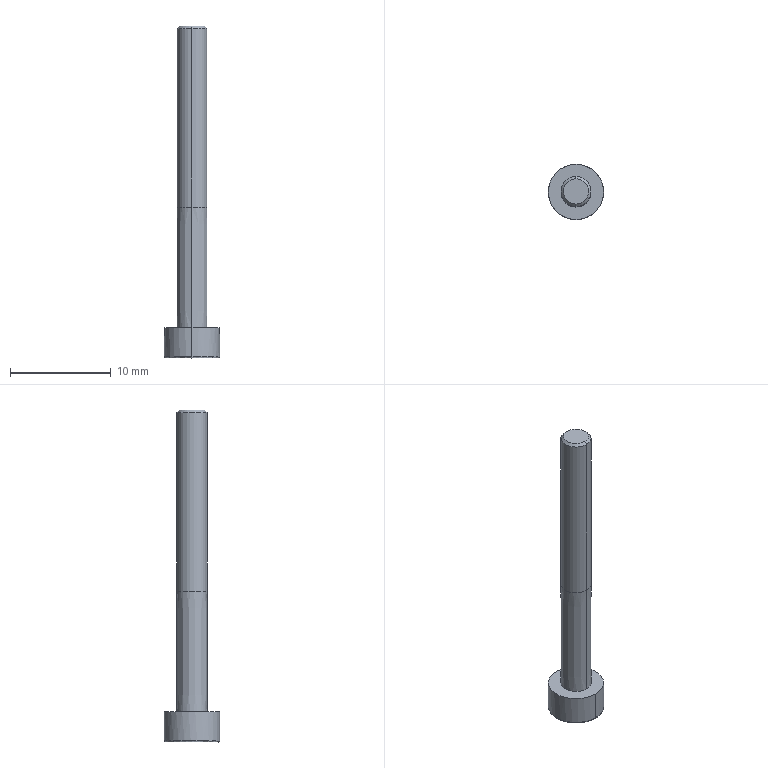Part | SolidWorks | features BaseBody 1 | 1 solid | 20 faces | box 5.5 x 5.5 x 33 mm | volume 275.938 mm3 | plane 10 | cylinder 4 | cone 4 | spline 2 | commonest cylinder face diameters 3 x2 5.5 x2
STEP:
#1=CARTESIAN_POINT('',(500.195,-28.804,245.644));
#2=VERTEX_POINT('',#1);
#3=CARTESIAN_POINT('',(502.224,-33.412,245.644));
#4=VERTEX_POINT('',#3);
#5=CARTESIAN_POINT('',(502.224,-30.662,245.644));
#6=DIRECTION('',(-0.000000001,-0.000000029,1.));
#7=DIRECTION('',(0.,-1.,-0.000000029));
#8=AXIS2_PLACEMENT_3D('',#5,#6,#7);
#9=CIRCLE('',#8,2.75);
#10=EDGE_CURVE('',#2,#4,#9,.T.);
#11=ORIENTED_EDGE('',*,*,#10,.F.);
#12=CARTESIAN_POINT('',(500.269,-28.872,245.544));
#13=VERTEX_POINT('',#12);
#14=CARTESIAN_POINT('',(500.269,-28.872,245.644));
#15=DIRECTION('',(-0.6753,-0.7375,-0.000000022));
#16=DIRECTION('',(-0.7375,0.6753,0.000000019));
#17=AXIS2_PLACEMENT_3D('',#14,#15,#16);
#18=CIRCLE('',#17,0.1);
#19=EDGE_CURVE('',#2,#13,#18,.T.);
#20=ORIENTED_EDGE('',*,*,#19,.T.);
#21=CARTESIAN_POINT('',(504.178,-32.451,245.544));
#22=VERTEX_POINT('',#21);
#23=CARTESIAN_POINT('',(500.269,-28.872,245.544));
#24=CARTESIAN_POINT('',(496.69,-32.781,245.544));
#25=CARTESIAN_POINT('',(500.599,-36.36,245.544));
#26=CARTESIAN_POINT('',(504.178,-32.451,245.544));
#27=(BOUNDED_CURVE()B_SPLINE_CURVE(3,(#23,#24,#25,#26),.UNSPECIFIED.,.F.,.F.)B_SPLINE_CURVE_WITH_KNOTS((4,4),(0.,1.),.UNSPECIFIED.)CURVE()GEOMETRIC_REPRESENTATION_ITEM()RATIONAL_B_SPLINE_CURVE((1.,0.3333,0.3333,1.))REPRESENTATION_ITEM(''));
#28=EDGE_CURVE('',#13,#22,#27,.T.);
#29=ORIENTED_EDGE('',*,*,#28,.T.);
#30=CARTESIAN_POINT('',(504.252,-32.519,245.644));
#31=VERTEX_POINT('',#30);
#32=CARTESIAN_POINT('',(504.178,-32.451,245.644));
#33=DIRECTION('',(0.6753,0.7375,0.000000022));
#34=DIRECTION('',(0.7375,-0.6753,-0.000000019));
#35=AXIS2_PLACEMENT_3D('',#32,#33,#34);
#36=CIRCLE('',#35,0.1);
#37=EDGE_CURVE('',#31,#22,#36,.T.);
#38=ORIENTED_EDGE('',*,*,#37,.F.);
#39=CARTESIAN_POINT('',(502.224,-30.662,245.644));
#40=DIRECTION('',(-0.000000001,-0.000000029,1.));
#41=DIRECTION('',(0.,-1.,-0.000000029));
#42=AXIS2_PLACEMENT_3D('',#39,#40,#41);
#43=CIRCLE('',#42,2.75);
#44=EDGE_CURVE('',#4,#31,#43,.T.);
#45=ORIENTED_EDGE('',*,*,#44,.F.);
#46=EDGE_LOOP('',(#11,#20,#29,#38,#45));
#47=FACE_OUTER_BOUND('',#46,.T.);
#48=CARTESIAN_POINT('',(500.195,-28.804,245.644));
#49=CARTESIAN_POINT('',(496.481,-32.861,245.644));
#50=CARTESIAN_POINT('',(500.537,-36.575,245.644));
#51=CARTESIAN_POINT('',(504.252,-32.519,245.644));
#52=CARTESIAN_POINT('',(500.195,-28.804,245.586));
#53=CARTESIAN_POINT('',(496.481,-32.861,245.586));
#54=CARTESIAN_POINT('',(500.537,-36.575,245.586));
#55=CARTESIAN_POINT('',(504.252,-32.519,245.586));
#56=CARTESIAN_POINT('',(500.226,-28.832,245.544));
#57=CARTESIAN_POINT('',(496.568,-32.828,245.544));
#58=CARTESIAN_POINT('',(500.563,-36.486,245.544));
#59=CARTESIAN_POINT('',(504.221,-32.491,245.544));
#60=CARTESIAN_POINT('',(500.269,-28.872,245.544));
#61=CARTESIAN_POINT('',(496.69,-32.781,245.544));
#62=CARTESIAN_POINT('',(500.599,-36.36,245.544));
#63=CARTESIAN_POINT('',(504.178,-32.451,245.544));
#64=(BOUNDED_SURFACE()B_SPLINE_SURFACE(3,3,((#48,#49,#50,#51),(#52,#53,#54,#55),(#56,#57,#58,#59),(#60,#61,#62,#63)),.UNSPECIFIED.,.F.,.F.,.F.)B_SPLINE_SURFACE_WITH_KNOTS((4,4),(4,4),(0.,1.),(0.,1.),.UNSPECIFIED.)GEOMETRIC_REPRESENTATION_ITEM()RATIONAL_B_SPLINE_SURFACE(((1.,0.3333,0.3333,1.),(0.8047,0.2682,0.2682,0.8047),(0.8047,0.2682,0.2682,0.8047),(1.,0.3333,0.3333,1.)))REPRESENTATION_ITEM('')SURFACE());
#65=ADVANCED_FACE('',(#47),#64,.T.);
#66=CARTESIAN_POINT('',(502.224,-32.162,260.544));
#67=VERTEX_POINT('',#66);
#68=CARTESIAN_POINT('',(502.224,-29.162,260.544));
#69=VERTEX_POINT('',#68);
#70=CARTESIAN_POINT('',(502.224,-30.662,260.544));
#71=DIRECTION('',(-0.000000001,-0.000000029,1.));
#72=DIRECTION('',(0.,-1.,-0.000000029));
#73=AXIS2_PLACEMENT_3D('',#70,#71,#72);
#74=CIRCLE('',#73,1.5);
#75=EDGE_CURVE('',#67,#69,#74,.T.);
#76=ORIENTED_EDGE('',*,*,#75,.T.);
#77=CARTESIAN_POINT('',(502.224,-29.162,278.294));
#78=VERTEX_POINT('',#77);
#79=CARTESIAN_POINT('',(502.224,-29.162,269.419));
#80=DIRECTION('',(-0.000000001,-0.000000029,1.));
#81=VECTOR('',#80,1000.);
#82=LINE('',#79,#81);
#83=EDGE_CURVE('',#69,#78,#82,.T.);
#84=ORIENTED_EDGE('',*,*,#83,.T.);
#85=CARTESIAN_POINT('',(502.224,-32.162,278.294));
#86=VERTEX_POINT('',#85);
#87=CARTESIAN_POINT('',(502.224,-30.662,278.294));
#88=DIRECTION('',(0.000000001,0.000000029,-1.));
#89=DIRECTION('',(0.,-1.,-0.000000029));
#90=AXIS2_PLACEMENT_3D('',#87,#88,#89);
#91=CIRCLE('',#90,1.5);
#92=EDGE_CURVE('',#78,#86,#91,.T.);
#93=ORIENTED_EDGE('',*,*,#92,.T.);
#94=CARTESIAN_POINT('',(502.224,-32.162,269.419));
#95=DIRECTION('',(-0.000000001,-0.000000029,1.));
#96=VECTOR('',#95,1000.);
#97=LINE('',#94,#96);
#98=EDGE_CURVE('',#67,#86,#97,.T.);
#99=ORIENTED_EDGE('',*,*,#98,.F.);
#100=EDGE_LOOP('',(#76,#84,#93,#99));
#101=FACE_OUTER_BOUND('',#100,.T.);
#102=CARTESIAN_POINT('',(502.224,-30.662,269.419));
#103=DIRECTION('',(-0.000000001,-0.000000029,1.));
#104=DIRECTION('',(0.,-1.,-0.000000029));
#105=AXIS2_PLACEMENT_3D('',#102,#103,#104);
#106=CYLINDRICAL_SURFACE('',#105,1.5);
#107=ADVANCED_FACE('',(#101),#106,.T.);
#108=CARTESIAN_POINT('',(502.224,-32.161,248.544));
#109=VERTEX_POINT('',#108);
#110=CARTESIAN_POINT('',(502.224,-29.162,248.544));
#111=VERTEX_POINT('',#110);
#112=CARTESIAN_POINT('',(502.224,-30.662,248.544));
#113=DIRECTION('',(-0.000000001,-0.000000029,1.));
#114=DIRECTION('',(0.,-1.,-0.000000029));
#115=AXIS2_PLACEMENT_3D('',#112,#113,#114);
#116=CIRCLE('',#115,1.499);
#117=EDGE_CURVE('',#109,#111,#116,.T.);
#118=ORIENTED_EDGE('',*,*,#117,.T.);
#119=CARTESIAN_POINT('',(502.224,-29.162,260.544));
#120=DIRECTION('',(-0.000000001,0.00006247,1.));
#121=VECTOR('',#120,1000.);
#122=LINE('',#119,#121);
#123=EDGE_CURVE('',#111,#69,#122,.T.);
#124=ORIENTED_EDGE('',*,*,#123,.T.);
#125=ORIENTED_EDGE('',*,*,#75,.F.);
#126=CARTESIAN_POINT('',(502.224,-32.162,260.544));
#127=DIRECTION('',(-0.000000001,-0.00006253,1.));
#128=VECTOR('',#127,1000.);
#129=LINE('',#126,#128);
#130=EDGE_CURVE('',#109,#67,#129,.T.);
#131=ORIENTED_EDGE('',*,*,#130,.F.);
#132=EDGE_LOOP('',(#118,#124,#125,#131));
#133=FACE_OUTER_BOUND('',#132,.T.);
#134=CARTESIAN_POINT('',(502.224,-30.662,260.544));
#135=DIRECTION('',(-0.000000001,-0.000000029,1.));
#136=DIRECTION('',(0.,-1.,-0.000000029));
#137=AXIS2_PLACEMENT_3D('',#134,#135,#136);
#138=CONICAL_SURFACE('',#137,1.5,0.0000625);
#139=ADVANCED_FACE('',(#133),#138,.T.);
#140=CARTESIAN_POINT('',(502.224,-29.412,278.544));
#141=VERTEX_POINT('',#140);
#142=CARTESIAN_POINT('',(502.224,-31.912,278.544));
#143=VERTEX_POINT('',#142);
#144=CARTESIAN_POINT('',(502.224,-30.662,278.544));
#145=DIRECTION('',(0.000000001,0.000000029,-1.));
#146=DIRECTION('',(0.,1.,0.000000029));
#147=AXIS2_PLACEMENT_3D('',#144,#145,#146);
#148=CIRCLE('',#147,1.25);
#149=EDGE_CURVE('',#141,#143,#148,.T.);
#150=ORIENTED_EDGE('',*,*,#149,.T.);
#151=CARTESIAN_POINT('',(502.224,-32.162,278.294));
#152=DIRECTION('',(0.,-0.7071,-0.7071));
#153=VECTOR('',#152,1000.);
#154=LINE('',#151,#153);
#155=EDGE_CURVE('',#143,#86,#154,.T.);
#156=ORIENTED_EDGE('',*,*,#155,.T.);
#157=ORIENTED_EDGE('',*,*,#92,.F.);
#158=CARTESIAN_POINT('',(502.224,-29.162,278.294));
#159=DIRECTION('',(0.,0.7071,-0.7071));
#160=VECTOR('',#159,1000.);
#161=LINE('',#158,#160);
#162=EDGE_CURVE('',#141,#78,#161,.T.);
#163=ORIENTED_EDGE('',*,*,#162,.F.);
#164=EDGE_LOOP('',(#150,#156,#157,#163));
#165=FACE_OUTER_BOUND('',#164,.T.);
#166=CARTESIAN_POINT('',(502.224,-30.662,278.294));
#167=DIRECTION('',(0.000000001,0.000000029,-1.));
#168=DIRECTION('',(0.,1.,0.000000029));
#169=AXIS2_PLACEMENT_3D('',#166,#167,#168);
#170=CONICAL_SURFACE('',#169,1.5,0.7854);
#171=ADVANCED_FACE('',(#165),#170,.T.);
#172=ORIENTED_EDGE('',*,*,#44,.T.);
#173=CARTESIAN_POINT('',(502.224,-27.912,245.644));
#174=VERTEX_POINT('',#173);
#175=CARTESIAN_POINT('',(502.224,-30.662,245.644));
#176=DIRECTION('',(-0.000000001,-0.000000029,1.));
#177=DIRECTION('',(0.,-1.,-0.000000029));
#178=AXIS2_PLACEMENT_3D('',#175,#176,#177);
#179=CIRCLE('',#178,2.75);
#180=EDGE_CURVE('',#31,#174,#179,.T.);
#181=ORIENTED_EDGE('',*,*,#180,.T.);
#182=CARTESIAN_POINT('',(502.224,-27.912,248.544));
#183=VERTEX_POINT('',#182);
#184=CARTESIAN_POINT('',(502.224,-27.912,247.094));
#185=DIRECTION('',(-0.000000001,-0.000000029,1.));
#186=VECTOR('',#185,1000.);
#187=LINE('',#184,#186);
#188=EDGE_CURVE('',#174,#183,#187,.T.);
#189=ORIENTED_EDGE('',*,*,#188,.T.);
#190=CARTESIAN_POINT('',(502.224,-33.412,248.544));
#191=VERTEX_POINT('',#190);
#192=CARTESIAN_POINT('',(502.224,-30.662,248.544));
#193=DIRECTION('',(-0.000000001,-0.000000029,1.));
#194=DIRECTION('',(0.,-1.,-0.000000029));
#195=AXIS2_PLACEMENT_3D('',#192,#193,#194);
#196=CIRCLE('',#195,2.75);
#197=EDGE_CURVE('',#191,#183,#196,.T.);
#198=ORIENTED_EDGE('',*,*,#197,.F.);
#199=CARTESIAN_POINT('',(502.224,-33.412,247.094));
#200=DIRECTION('',(-0.000000001,-0.000000029,1.));
#201=VECTOR('',#200,1000.);
#202=LINE('',#199,#201);
#203=EDGE_CURVE('',#4,#191,#202,.T.);
#204=ORIENTED_EDGE('',*,*,#203,.F.);
#205=EDGE_LOOP('',(#172,#181,#189,#198,#204));
#206=FACE_OUTER_BOUND('',#205,.T.);
#207=CARTESIAN_POINT('',(502.224,-30.662,247.094));
#208=DIRECTION('',(-0.000000001,-0.000000029,1.));
#209=DIRECTION('',(0.,-1.,-0.000000029));
#210=AXIS2_PLACEMENT_3D('',#207,#208,#209);
#211=CYLINDRICAL_SURFACE('',#210,2.75);
#212=ADVANCED_FACE('',(#206),#211,.T.);
#213=ORIENTED_EDGE('',*,*,#83,.F.);
#214=CARTESIAN_POINT('',(502.224,-30.662,260.544));
#215=DIRECTION('',(-0.000000001,-0.000000029,1.));
#216=DIRECTION('',(0.,-1.,-0.000000029));
#217=AXIS2_PLACEMENT_3D('',#214,#215,#216);
#218=CIRCLE('',#217,1.5);
#219=EDGE_CURVE('',#69,#67,#218,.T.);
#220=ORIENTED_EDGE('',*,*,#219,.T.);
#221=ORIENTED_EDGE('',*,*,#98,.T.);
#222=CARTESIAN_POINT('',(502.224,-30.662,278.294));
#223=DIRECTION('',(0.000000001,0.000000029,-1.));
#224=DIRECTION('',(0.,-1.,-0.000000029));
#225=AXIS2_PLACEMENT_3D('',#222,#223,#224);
#226=CIRCLE('',#225,1.5);
#227=EDGE_CURVE('',#86,#78,#226,.T.);
#228=ORIENTED_EDGE('',*,*,#227,.T.);
#229=EDGE_LOOP('',(#213,#220,#221,#228));
#230=FACE_OUTER_BOUND('',#229,.T.);
#231=CARTESIAN_POINT('',(502.224,-30.662,269.419));
#232=DIRECTION('',(-0.000000001,-0.000000029,1.));
#233=DIRECTION('',(0.,-1.,-0.000000029));
#234=AXIS2_PLACEMENT_3D('',#231,#232,#233);
#235=CYLINDRICAL_SURFACE('',#234,1.5);
#236=ADVANCED_FACE('',(#230),#235,.T.);
#237=ORIENTED_EDGE('',*,*,#123,.F.);
#238=CARTESIAN_POINT('',(502.224,-30.662,248.544));
#239=DIRECTION('',(-0.000000001,-0.000000029,1.));
#240=DIRECTION('',(0.,-1.,-0.000000029));
#241=AXIS2_PLACEMENT_3D('',#238,#239,#240);
#242=CIRCLE('',#241,1.499);
#243=EDGE_CURVE('',#111,#109,#242,.T.);
#244=ORIENTED_EDGE('',*,*,#243,.T.);
#245=ORIENTED_EDGE('',*,*,#130,.T.);
#246=ORIENTED_EDGE('',*,*,#219,.F.);
#247=EDGE_LOOP('',(#237,#244,#245,#246));
#248=FACE_OUTER_BOUND('',#247,.T.);
#249=CARTESIAN_POINT('',(502.224,-30.662,260.544));
#250=DIRECTION('',(-0.000000001,-0.000000029,1.));
#251=DIRECTION('',(0.,-1.,-0.000000029));
#252=AXIS2_PLACEMENT_3D('',#249,#250,#251);
#253=CONICAL_SURFACE('',#252,1.5,0.0000625);
#254=ADVANCED_FACE('',(#248),#253,.T.);
#255=ORIENTED_EDGE('',*,*,#155,.F.);
#256=CARTESIAN_POINT('',(502.224,-30.662,278.544));
#257=DIRECTION('',(0.000000001,0.000000029,-1.));
#258=DIRECTION('',(0.,1.,0.000000029));
#259=AXIS2_PLACEMENT_3D('',#256,#257,#258);
#260=CIRCLE('',#259,1.25);
#261=EDGE_CURVE('',#143,#141,#260,.T.);
#262=ORIENTED_EDGE('',*,*,#261,.T.);
#263=ORIENTED_EDGE('',*,*,#162,.T.);
#264=ORIENTED_EDGE('',*,*,#227,.F.);
#265=EDGE_LOOP('',(#255,#262,#263,#264));
#266=FACE_OUTER_BOUND('',#265,.T.);
#267=CARTESIAN_POINT('',(502.224,-30.662,278.294));
#268=DIRECTION('',(0.000000001,0.000000029,-1.));
#269=DIRECTION('',(0.,1.,0.000000029));
#270=AXIS2_PLACEMENT_3D('',#267,#268,#269);
#271=CONICAL_SURFACE('',#270,1.5,0.7854);
#272=ADVANCED_FACE('',(#266),#271,.T.);
#273=ORIENTED_EDGE('',*,*,#117,.F.);
#274=ORIENTED_EDGE('',*,*,#243,.F.);
#275=EDGE_LOOP('',(#273,#274));
#276=FACE_BOUND('',#275,.T.);
#277=ORIENTED_EDGE('',*,*,#197,.T.);
#278=CARTESIAN_POINT('',(502.224,-30.662,248.544));
#279=DIRECTION('',(-0.000000001,-0.000000029,1.));
#280=DIRECTION('',(0.,-1.,-0.000000029));
#281=AXIS2_PLACEMENT_3D('',#278,#279,#280);
#282=CIRCLE('',#281,2.75);
#283=EDGE_CURVE('',#183,#191,#282,.T.);
#284=ORIENTED_EDGE('',*,*,#283,.T.);
#285=EDGE_LOOP('',(#277,#284));
#286=FACE_OUTER_BOUND('',#285,.T.);
#287=CARTESIAN_POINT('',(503.238,-31.59,248.544));
#288=DIRECTION('',(-0.000000001,-0.000000029,1.));
#289=DIRECTION('',(0.,-1.,-0.000000029));
#290=AXIS2_PLACEMENT_3D('',#287,#288,#289);
#291=PLANE('',#290);
#292=ADVANCED_FACE('',(#276,#286),#291,.T.);
#293=ORIENTED_EDGE('',*,*,#149,.F.);
#294=ORIENTED_EDGE('',*,*,#261,.F.);
#295=EDGE_LOOP('',(#293,#294));
#296=FACE_OUTER_BOUND('',#295,.T.);
#297=CARTESIAN_POINT('',(502.684,-31.084,278.544));
#298=DIRECTION('',(-0.000000001,-0.000000029,1.));
#299=DIRECTION('',(0.,-1.,-0.000000029));
#300=AXIS2_PLACEMENT_3D('',#297,#298,#299);
#301=PLANE('',#300);
#302=ADVANCED_FACE('',(#296),#301,.T.);
#303=ORIENTED_EDGE('',*,*,#188,.F.);
#304=CARTESIAN_POINT('',(502.224,-30.662,245.644));
#305=DIRECTION('',(-0.000000001,-0.000000029,1.));
#306=DIRECTION('',(0.,-1.,-0.000000029));
#307=AXIS2_PLACEMENT_3D('',#304,#305,#306);
#308=CIRCLE('',#307,2.75);
#309=EDGE_CURVE('',#174,#2,#308,.T.);
#310=ORIENTED_EDGE('',*,*,#309,.T.);
#311=ORIENTED_EDGE('',*,*,#10,.T.);
#312=ORIENTED_EDGE('',*,*,#203,.T.);
#313=ORIENTED_EDGE('',*,*,#283,.F.);
#314=EDGE_LOOP('',(#303,#310,#311,#312,#313));
#315=FACE_OUTER_BOUND('',#314,.T.);
#316=CARTESIAN_POINT('',(502.224,-30.662,247.094));
#317=DIRECTION('',(-0.000000001,-0.000000029,1.));
#318=DIRECTION('',(0.,-1.,-0.000000029));
#319=AXIS2_PLACEMENT_3D('',#316,#317,#318);
#320=CYLINDRICAL_SURFACE('',#319,2.75);
#321=ADVANCED_FACE('',(#315),#320,.T.);
#322=ORIENTED_EDGE('',*,*,#19,.F.);
#323=ORIENTED_EDGE('',*,*,#309,.F.);
#324=ORIENTED_EDGE('',*,*,#180,.F.);
#325=ORIENTED_EDGE('',*,*,#37,.T.);
#326=CARTESIAN_POINT('',(504.178,-32.451,245.544));
#327=CARTESIAN_POINT('',(507.757,-28.542,245.544));
#328=CARTESIAN_POINT('',(503.848,-24.963,245.544));
#329=CARTESIAN_POINT('',(500.269,-28.872,245.544));
#330=(BOUNDED_CURVE()B_SPLINE_CURVE(3,(#326,#327,#328,#329),.UNSPECIFIED.,.F.,.T.)B_SPLINE_CURVE_WITH_KNOTS((4,4),(0.,1.),.UNSPECIFIED.)CURVE()GEOMETRIC_REPRESENTATION_ITEM()RATIONAL_B_SPLINE_CURVE((1.,0.3333,0.3333,1.))REPRESENTATION_ITEM(''));
#331=EDGE_CURVE('',#22,#13,#330,.T.);
#332=ORIENTED_EDGE('',*,*,#331,.T.);
#333=EDGE_LOOP('',(#322,#323,#324,#325,#332));
#334=FACE_OUTER_BOUND('',#333,.T.);
#335=CARTESIAN_POINT('',(504.252,-32.519,245.644));
#336=CARTESIAN_POINT('',(507.966,-28.462,245.644));
#337=CARTESIAN_POINT('',(503.91,-24.748,245.644));
#338=CARTESIAN_POINT('',(500.195,-28.804,245.644));
#339=CARTESIAN_POINT('',(504.252,-32.519,245.586));
#340=CARTESIAN_POINT('',(507.966,-28.462,245.586));
#341=CARTESIAN_POINT('',(503.91,-24.748,245.586));
#342=CARTESIAN_POINT('',(500.195,-28.804,245.586));
#343=CARTESIAN_POINT('',(504.221,-32.491,245.544));
#344=CARTESIAN_POINT('',(507.88,-28.496,245.544));
#345=CARTESIAN_POINT('',(503.884,-24.837,245.544));
#346=CARTESIAN_POINT('',(500.226,-28.832,245.544));
#347=CARTESIAN_POINT('',(504.178,-32.451,245.544));
#348=CARTESIAN_POINT('',(507.757,-28.542,245.544));
#349=CARTESIAN_POINT('',(503.848,-24.963,245.544));
#350=CARTESIAN_POINT('',(500.269,-28.872,245.544));
#351=(BOUNDED_SURFACE()B_SPLINE_SURFACE(3,3,((#335,#336,#337,#338),(#339,#340,#341,#342),(#343,#344,#345,#346),(#347,#348,#349,#350)),.UNSPECIFIED.,.F.,.F.,.F.)B_SPLINE_SURFACE_WITH_KNOTS((4,4),(4,4),(0.,1.),(0.,1.),.UNSPECIFIED.)GEOMETRIC_REPRESENTATION_ITEM()RATIONAL_B_SPLINE_SURFACE(((1.,0.3333,0.3333,1.),(0.8047,0.2682,0.2682,0.8047),(0.8047,0.2682,0.2682,0.8047),(1.,0.3333,0.3333,1.)))REPRESENTATION_ITEM('')SURFACE());
#352=ADVANCED_FACE('',(#334),#351,.T.);
#353=ORIENTED_EDGE('',*,*,#28,.F.);
#354=ORIENTED_EDGE('',*,*,#331,.F.);
#355=EDGE_LOOP('',(#353,#354));
#356=FACE_OUTER_BOUND('',#355,.T.);
#357=CARTESIAN_POINT('',(502.535,-29.252,245.544));
#358=VERTEX_POINT('',#357);
#359=CARTESIAN_POINT('',(501.159,-29.687,245.544));
#360=VERTEX_POINT('',#359);
#361=CARTESIAN_POINT('',(502.535,-29.252,245.544));
#362=DIRECTION('',(-0.9536,-0.301,-0.000000009));
#363=VECTOR('',#362,1000.);
#364=LINE('',#361,#363);
#365=EDGE_CURVE('',#358,#360,#364,.T.);
#366=ORIENTED_EDGE('',*,*,#365,.T.);
#367=CARTESIAN_POINT('',(500.847,-31.096,245.544));
#368=VERTEX_POINT('',#367);
#369=CARTESIAN_POINT('',(501.159,-29.687,245.544));
#370=DIRECTION('',(-0.2161,-0.9764,-0.000000028));
#371=VECTOR('',#370,1000.);
#372=LINE('',#369,#371);
#373=EDGE_CURVE('',#360,#368,#372,.T.);
#374=ORIENTED_EDGE('',*,*,#373,.T.);
#375=CARTESIAN_POINT('',(501.912,-32.071,245.544));
#376=VERTEX_POINT('',#375);
#377=CARTESIAN_POINT('',(500.847,-31.096,245.544));
#378=DIRECTION('',(0.7375,-0.6753,-0.000000019));
#379=VECTOR('',#378,1000.);
#380=LINE('',#377,#379);
#381=EDGE_CURVE('',#368,#376,#380,.T.);
#382=ORIENTED_EDGE('',*,*,#381,.T.);
#383=CARTESIAN_POINT('',(503.288,-31.636,245.544));
#384=VERTEX_POINT('',#383);
#385=CARTESIAN_POINT('',(501.912,-32.071,245.544));
#386=DIRECTION('',(0.9536,0.301,0.000000009));
#387=VECTOR('',#386,1000.);
#388=LINE('',#385,#387);
#389=EDGE_CURVE('',#376,#384,#388,.T.);
#390=ORIENTED_EDGE('',*,*,#389,.T.);
#391=CARTESIAN_POINT('',(503.6,-30.227,245.544));
#392=VERTEX_POINT('',#391);
#393=CARTESIAN_POINT('',(503.288,-31.636,245.544));
#394=DIRECTION('',(0.2161,0.9764,0.000000028));
#395=VECTOR('',#394,1000.);
#396=LINE('',#393,#395);
#397=EDGE_CURVE('',#384,#392,#396,.T.);
#398=ORIENTED_EDGE('',*,*,#397,.T.);
#399=CARTESIAN_POINT('',(503.6,-30.227,245.544));
#400=DIRECTION('',(-0.7375,0.6753,0.000000019));
#401=VECTOR('',#400,1000.);
#402=LINE('',#399,#401);
#403=EDGE_CURVE('',#392,#358,#402,.T.);
#404=ORIENTED_EDGE('',*,*,#403,.T.);
#405=EDGE_LOOP('',(#366,#374,#382,#390,#398,#404));
#406=FACE_BOUND('',#405,.T.);
#407=CARTESIAN_POINT('',(503.201,-31.556,245.544));
#408=DIRECTION('',(0.000000001,0.000000029,-1.));
#409=DIRECTION('',(0.,1.,0.000000029));
#410=AXIS2_PLACEMENT_3D('',#407,#408,#409);
#411=PLANE('',#410);
#412=ADVANCED_FACE('',(#356,#406),#411,.T.);
#413=CARTESIAN_POINT('',(500.847,-31.096,246.844));
#414=VERTEX_POINT('',#413);
#415=CARTESIAN_POINT('',(500.847,-31.096,245.544));
#416=DIRECTION('',(0.000000005,-0.000000001,1.));
#417=VECTOR('',#416,1000.);
#418=LINE('',#415,#417);
#419=EDGE_CURVE('',#368,#414,#418,.T.);
#420=ORIENTED_EDGE('',*,*,#419,.F.);
#421=ORIENTED_EDGE('',*,*,#373,.F.);
#422=CARTESIAN_POINT('',(501.159,-29.687,246.844));
#423=VERTEX_POINT('',#422);
#424=CARTESIAN_POINT('',(501.159,-29.687,245.544));
#425=DIRECTION('',(-0.000000005,0.000000001,-1.));
#426=VECTOR('',#425,1000.);
#427=LINE('',#424,#426);
#428=EDGE_CURVE('',#423,#360,#427,.T.);
#429=ORIENTED_EDGE('',*,*,#428,.F.);
#430=CARTESIAN_POINT('',(500.847,-31.096,246.844));
#431=DIRECTION('',(0.2161,0.9764,0.));
#432=VECTOR('',#431,1000.);
#433=LINE('',#430,#432);
#434=EDGE_CURVE('',#414,#423,#433,.T.);
#435=ORIENTED_EDGE('',*,*,#434,.F.);
#436=EDGE_LOOP('',(#420,#421,#429,#435));
#437=FACE_OUTER_BOUND('',#436,.T.);
#438=CARTESIAN_POINT('',(500.847,-31.096,245.544));
#439=DIRECTION('',(-0.9764,0.2161,0.000000006));
#440=DIRECTION('',(-0.2161,-0.9764,0.));
#441=AXIS2_PLACEMENT_3D('',#438,#439,#440);
#442=PLANE('',#441);
#443=ADVANCED_FACE('',(#437),#442,.F.);
#444=ORIENTED_EDGE('',*,*,#428,.T.);
#445=ORIENTED_EDGE('',*,*,#365,.F.);
#446=CARTESIAN_POINT('',(502.535,-29.252,246.844));
#447=VERTEX_POINT('',#446);
#448=CARTESIAN_POINT('',(502.535,-29.252,245.544));
#449=DIRECTION('',(-0.000000008,0.000000026,-1.));
#450=VECTOR('',#449,1000.);
#451=LINE('',#448,#450);
#452=EDGE_CURVE('',#447,#358,#451,.T.);
#453=ORIENTED_EDGE('',*,*,#452,.F.);
#454=CARTESIAN_POINT('',(501.159,-29.687,246.844));
#455=DIRECTION('',(0.9536,0.301,0.));
#456=VECTOR('',#455,1000.);
#457=LINE('',#454,#456);
#458=EDGE_CURVE('',#423,#447,#457,.T.);
#459=ORIENTED_EDGE('',*,*,#458,.F.);
#460=EDGE_LOOP('',(#444,#445,#453,#459));
#461=FACE_OUTER_BOUND('',#460,.T.);
#462=CARTESIAN_POINT('',(501.159,-29.687,245.544));
#463=DIRECTION('',(-0.301,0.9536,0.000000027));
#464=DIRECTION('',(-0.9536,-0.301,0.));
#465=AXIS2_PLACEMENT_3D('',#462,#463,#464);
#466=PLANE('',#465);
#467=ADVANCED_FACE('',(#461),#466,.F.);
#468=ORIENTED_EDGE('',*,*,#452,.T.);
#469=ORIENTED_EDGE('',*,*,#403,.F.);
#470=CARTESIAN_POINT('',(503.6,-30.227,246.844));
#471=VERTEX_POINT('',#470);
#472=CARTESIAN_POINT('',(503.6,-30.227,245.544));
#473=DIRECTION('',(0.000000015,0.000000016,-1.));
#474=VECTOR('',#473,1000.);
#475=LINE('',#472,#474);
#476=EDGE_CURVE('',#471,#392,#475,.T.);
#477=ORIENTED_EDGE('',*,*,#476,.F.);
#478=CARTESIAN_POINT('',(502.535,-29.252,246.844));
#479=DIRECTION('',(0.7375,-0.6753,0.));
#480=VECTOR('',#479,1000.);
#481=LINE('',#478,#480);
#482=EDGE_CURVE('',#447,#471,#481,.T.);
#483=ORIENTED_EDGE('',*,*,#482,.F.);
#484=EDGE_LOOP('',(#468,#469,#477,#483));
#485=FACE_OUTER_BOUND('',#484,.T.);
#486=CARTESIAN_POINT('',(502.535,-29.252,245.544));
#487=DIRECTION('',(0.6753,0.7375,0.000000022));
#488=DIRECTION('',(-0.7375,0.6753,0.));
#489=AXIS2_PLACEMENT_3D('',#486,#487,#488);
#490=PLANE('',#489);
#491=ADVANCED_FACE('',(#485),#490,.F.);
#492=ORIENTED_EDGE('',*,*,#476,.T.);
#493=ORIENTED_EDGE('',*,*,#397,.F.);
#494=CARTESIAN_POINT('',(503.288,-31.636,246.844));
#495=VERTEX_POINT('',#494);
#496=CARTESIAN_POINT('',(503.288,-31.636,245.544));
#497=DIRECTION('',(-0.000000005,0.000000001,-1.));
#498=VECTOR('',#497,1000.);
#499=LINE('',#496,#498);
#500=EDGE_CURVE('',#495,#384,#499,.T.);
#501=ORIENTED_EDGE('',*,*,#500,.F.);
#502=CARTESIAN_POINT('',(503.6,-30.227,246.844));
#503=DIRECTION('',(-0.2161,-0.9764,0.));
#504=VECTOR('',#503,1000.);
#505=LINE('',#502,#504);
#506=EDGE_CURVE('',#471,#495,#505,.T.);
#507=ORIENTED_EDGE('',*,*,#506,.F.);
#508=EDGE_LOOP('',(#492,#493,#501,#507));
#509=FACE_OUTER_BOUND('',#508,.T.);
#510=CARTESIAN_POINT('',(503.6,-30.227,245.544));
#511=DIRECTION('',(0.9764,-0.2161,-0.000000006));
#512=DIRECTION('',(0.2161,0.9764,0.));
#513=AXIS2_PLACEMENT_3D('',#510,#511,#512);
#514=PLANE('',#513);
#515=ADVANCED_FACE('',(#509),#514,.F.);
#516=ORIENTED_EDGE('',*,*,#500,.T.);
#517=ORIENTED_EDGE('',*,*,#389,.F.);
#518=CARTESIAN_POINT('',(501.912,-32.071,246.844));
#519=VERTEX_POINT('',#518);
#520=CARTESIAN_POINT('',(501.912,-32.071,245.544));
#521=DIRECTION('',(-0.000000008,0.000000026,-1.));
#522=VECTOR('',#521,1000.);
#523=LINE('',#520,#522);
#524=EDGE_CURVE('',#519,#376,#523,.T.);
#525=ORIENTED_EDGE('',*,*,#524,.F.);
#526=CARTESIAN_POINT('',(503.288,-31.636,246.844));
#527=DIRECTION('',(-0.9536,-0.301,0.));
#528=VECTOR('',#527,1000.);
#529=LINE('',#526,#528);
#530=EDGE_CURVE('',#495,#519,#529,.T.);
#531=ORIENTED_EDGE('',*,*,#530,.F.);
#532=EDGE_LOOP('',(#516,#517,#525,#531));
#533=FACE_OUTER_BOUND('',#532,.T.);
#534=CARTESIAN_POINT('',(503.288,-31.636,245.544));
#535=DIRECTION('',(0.301,-0.9536,-0.000000027));
#536=DIRECTION('',(0.9536,0.301,0.));
#537=AXIS2_PLACEMENT_3D('',#534,#535,#536);
#538=PLANE('',#537);
#539=ADVANCED_FACE('',(#533),#538,.F.);
#540=ORIENTED_EDGE('',*,*,#524,.T.);
#541=ORIENTED_EDGE('',*,*,#381,.F.);
#542=ORIENTED_EDGE('',*,*,#419,.T.);
#543=CARTESIAN_POINT('',(501.912,-32.071,246.844));
#544=DIRECTION('',(-0.7375,0.6753,0.));
#545=VECTOR('',#544,1000.);
#546=LINE('',#543,#545);
#547=EDGE_CURVE('',#519,#414,#546,.T.);
#548=ORIENTED_EDGE('',*,*,#547,.F.);
#549=EDGE_LOOP('',(#540,#541,#542,#548));
#550=FACE_OUTER_BOUND('',#549,.T.);
#551=CARTESIAN_POINT('',(501.912,-32.071,245.544));
#552=DIRECTION('',(-0.6753,-0.7375,-0.000000022));
#553=DIRECTION('',(0.7375,-0.6753,0.));
#554=AXIS2_PLACEMENT_3D('',#551,#552,#553);
#555=PLANE('',#554);
#556=ADVANCED_FACE('',(#550),#555,.F.);
#557=ORIENTED_EDGE('',*,*,#506,.T.);
#558=ORIENTED_EDGE('',*,*,#530,.T.);
#559=ORIENTED_EDGE('',*,*,#547,.T.);
#560=ORIENTED_EDGE('',*,*,#434,.T.);
#561=ORIENTED_EDGE('',*,*,#458,.T.);
#562=ORIENTED_EDGE('',*,*,#482,.T.);
#563=EDGE_LOOP('',(#557,#558,#559,#560,#561,#562));
#564=FACE_OUTER_BOUND('',#563,.T.);
#565=CARTESIAN_POINT('',(502.224,-30.662,246.844));
#566=DIRECTION('',(0.000000001,0.000000029,-1.));
#567=DIRECTION('',(0.,1.,0.000000029));
#568=AXIS2_PLACEMENT_3D('',#565,#566,#567);
#569=PLANE('',#568);
#570=ADVANCED_FACE('',(#564),#569,.T.);
#571=CLOSED_SHELL('',(#65,#107,#139,#171,#212,#236,#254,#272,#292,#302,#321,#352,#412,#443,#467,#491,#515,#539,#556,#570));
#572=MANIFOLD_SOLID_BREP('',#571);
#573=CARTESIAN_POINT('',(0.,0.,0.));
#574=DIRECTION('',(0.,0.,1.));
#575=DIRECTION('',(1.,0.,0.));
#576=AXIS2_PLACEMENT_3D('',#573,#574,#575);
#577=(LENGTH_UNIT()NAMED_UNIT(*)SI_UNIT(.MILLI.,.METRE.));
#578=UNCERTAINTY_MEASURE_WITH_UNIT(LENGTH_MEASURE(0.00001),#577,'','');
#579=(NAMED_UNIT(*)PLANE_ANGLE_UNIT()SI_UNIT($,.RADIAN.));
#580=(NAMED_UNIT(*)SI_UNIT($,.STERADIAN.)SOLID_ANGLE_UNIT());
#581=(GEOMETRIC_REPRESENTATION_CONTEXT(3)GLOBAL_UNCERTAINTY_ASSIGNED_CONTEXT((#578))GLOBAL_UNIT_ASSIGNED_CONTEXT((#577,#579,#580))REPRESENTATION_CONTEXT('',''));
#582=ADVANCED_BREP_SHAPE_REPRESENTATION('',(#572,#576),#581);